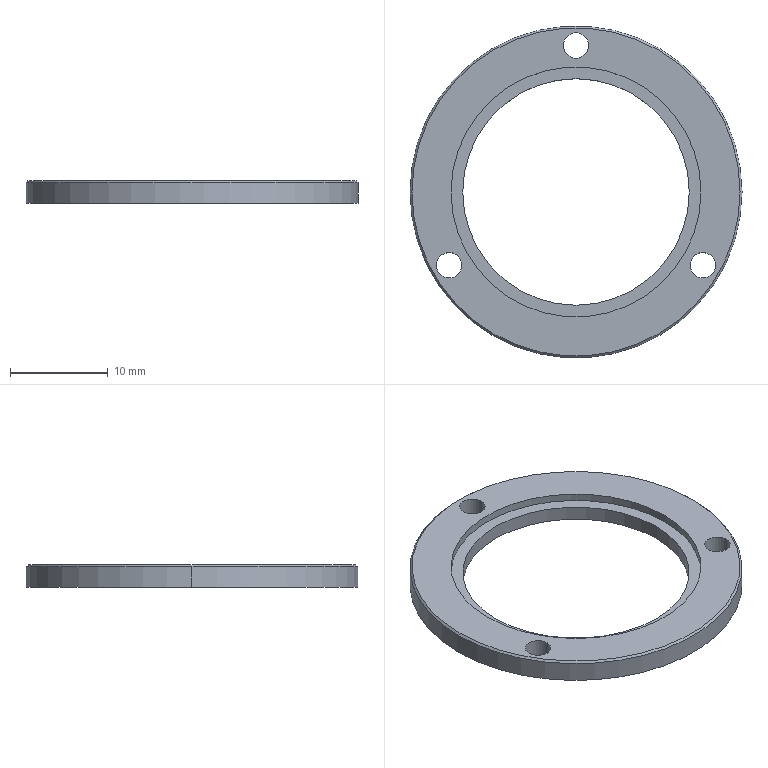Part | SolidWorks | features ICE 6, Chamfer 2, Cut 2, HoleWzd 2, MoveFace 2, Extrusion 1 | 1 solid | 17 faces | box 34 x 34 x 2.3 mm | volume 1004 mm3 | cylinder 12 | plane 3 | cone 2 | commonest cylinder face diameters 2.6 x6 23.2 x2 25.6 x2 34 x2
STEP:
#1=CARTESIAN_POINT('',(39.89,-35.7,-1.3));
#2=VERTEX_POINT('',#1);
#3=CARTESIAN_POINT('',(42.49,-35.7,-1.3));
#4=VERTEX_POINT('',#3);
#5=CARTESIAN_POINT('',(41.19,-35.7,-1.3));
#6=DIRECTION('',(0.,0.,1.));
#7=DIRECTION('',(1.,0.,0.));
#8=AXIS2_PLACEMENT_3D('',#5,#6,#7);
#9=CIRCLE('',#8,1.3);
#10=EDGE_CURVE('',#2,#4,#9,.T.);
#11=ORIENTED_EDGE('',*,*,#10,.F.);
#12=CARTESIAN_POINT('',(39.89,-35.7,1.));
#13=VERTEX_POINT('',#12);
#14=CARTESIAN_POINT('',(39.89,-35.7,-1.3));
#15=DIRECTION('',(0.,0.,1.));
#16=VECTOR('',#15,1000.);
#17=LINE('',#14,#16);
#18=EDGE_CURVE('',#2,#13,#17,.T.);
#19=ORIENTED_EDGE('',*,*,#18,.T.);
#20=CARTESIAN_POINT('',(42.49,-35.7,1.));
#21=VERTEX_POINT('',#20);
#22=CARTESIAN_POINT('',(41.19,-35.7,1.));
#23=DIRECTION('',(0.,0.,1.));
#24=DIRECTION('',(1.,0.,0.));
#25=AXIS2_PLACEMENT_3D('',#22,#23,#24);
#26=CIRCLE('',#25,1.3);
#27=EDGE_CURVE('',#13,#21,#26,.T.);
#28=ORIENTED_EDGE('',*,*,#27,.T.);
#29=CARTESIAN_POINT('',(42.49,-35.7,-1.3));
#30=DIRECTION('',(0.,0.,1.));
#31=VECTOR('',#30,1000.);
#32=LINE('',#29,#31);
#33=EDGE_CURVE('',#4,#21,#32,.T.);
#34=ORIENTED_EDGE('',*,*,#33,.F.);
#35=EDGE_LOOP('',(#11,#19,#28,#34));
#36=FACE_OUTER_BOUND('',#35,.T.);
#37=CARTESIAN_POINT('',(41.19,-35.7,-1.3));
#38=DIRECTION('',(0.,0.,1.));
#39=DIRECTION('',(1.,0.,0.));
#40=AXIS2_PLACEMENT_3D('',#37,#38,#39);
#41=CYLINDRICAL_SURFACE('',#40,1.3);
#42=ADVANCED_FACE('',(#36),#41,.F.);
#43=CARTESIAN_POINT('',(26.9,-13.2,-1.3));
#44=VERTEX_POINT('',#43);
#45=CARTESIAN_POINT('',(29.5,-13.2,-1.3));
#46=VERTEX_POINT('',#45);
#47=CARTESIAN_POINT('',(28.2,-13.2,-1.3));
#48=DIRECTION('',(0.,0.,1.));
#49=DIRECTION('',(1.,0.,0.));
#50=AXIS2_PLACEMENT_3D('',#47,#48,#49);
#51=CIRCLE('',#50,1.3);
#52=EDGE_CURVE('',#44,#46,#51,.T.);
#53=ORIENTED_EDGE('',*,*,#52,.F.);
#54=CARTESIAN_POINT('',(26.9,-13.2,1.));
#55=VERTEX_POINT('',#54);
#56=CARTESIAN_POINT('',(26.9,-13.2,-1.3));
#57=DIRECTION('',(0.,0.,1.));
#58=VECTOR('',#57,1000.);
#59=LINE('',#56,#58);
#60=EDGE_CURVE('',#44,#55,#59,.T.);
#61=ORIENTED_EDGE('',*,*,#60,.T.);
#62=CARTESIAN_POINT('',(29.5,-13.2,1.));
#63=VERTEX_POINT('',#62);
#64=CARTESIAN_POINT('',(28.2,-13.2,1.));
#65=DIRECTION('',(0.,0.,1.));
#66=DIRECTION('',(1.,0.,0.));
#67=AXIS2_PLACEMENT_3D('',#64,#65,#66);
#68=CIRCLE('',#67,1.3);
#69=EDGE_CURVE('',#55,#63,#68,.T.);
#70=ORIENTED_EDGE('',*,*,#69,.T.);
#71=CARTESIAN_POINT('',(29.5,-13.2,-1.3));
#72=DIRECTION('',(0.,0.,1.));
#73=VECTOR('',#72,1000.);
#74=LINE('',#71,#73);
#75=EDGE_CURVE('',#46,#63,#74,.T.);
#76=ORIENTED_EDGE('',*,*,#75,.F.);
#77=EDGE_LOOP('',(#53,#61,#70,#76));
#78=FACE_OUTER_BOUND('',#77,.T.);
#79=CARTESIAN_POINT('',(28.2,-13.2,-1.3));
#80=DIRECTION('',(0.,0.,1.));
#81=DIRECTION('',(1.,0.,0.));
#82=AXIS2_PLACEMENT_3D('',#79,#80,#81);
#83=CYLINDRICAL_SURFACE('',#82,1.3);
#84=ADVANCED_FACE('',(#78),#83,.F.);
#85=CARTESIAN_POINT('',(13.91,-35.7,-1.3));
#86=VERTEX_POINT('',#85);
#87=CARTESIAN_POINT('',(16.51,-35.7,-1.3));
#88=VERTEX_POINT('',#87);
#89=CARTESIAN_POINT('',(15.21,-35.7,-1.3));
#90=DIRECTION('',(0.,0.,1.));
#91=DIRECTION('',(1.,0.,0.));
#92=AXIS2_PLACEMENT_3D('',#89,#90,#91);
#93=CIRCLE('',#92,1.3);
#94=EDGE_CURVE('',#86,#88,#93,.T.);
#95=ORIENTED_EDGE('',*,*,#94,.F.);
#96=CARTESIAN_POINT('',(13.91,-35.7,1.));
#97=VERTEX_POINT('',#96);
#98=CARTESIAN_POINT('',(13.91,-35.7,-1.3));
#99=DIRECTION('',(0.,0.,1.));
#100=VECTOR('',#99,1000.);
#101=LINE('',#98,#100);
#102=EDGE_CURVE('',#86,#97,#101,.T.);
#103=ORIENTED_EDGE('',*,*,#102,.T.);
#104=CARTESIAN_POINT('',(16.51,-35.7,1.));
#105=VERTEX_POINT('',#104);
#106=CARTESIAN_POINT('',(15.21,-35.7,1.));
#107=DIRECTION('',(0.,0.,1.));
#108=DIRECTION('',(1.,0.,0.));
#109=AXIS2_PLACEMENT_3D('',#106,#107,#108);
#110=CIRCLE('',#109,1.3);
#111=EDGE_CURVE('',#97,#105,#110,.T.);
#112=ORIENTED_EDGE('',*,*,#111,.T.);
#113=CARTESIAN_POINT('',(16.51,-35.7,-1.3));
#114=DIRECTION('',(0.,0.,1.));
#115=VECTOR('',#114,1000.);
#116=LINE('',#113,#115);
#117=EDGE_CURVE('',#88,#105,#116,.T.);
#118=ORIENTED_EDGE('',*,*,#117,.F.);
#119=EDGE_LOOP('',(#95,#103,#112,#118));
#120=FACE_OUTER_BOUND('',#119,.T.);
#121=CARTESIAN_POINT('',(15.21,-35.7,-1.3));
#122=DIRECTION('',(0.,0.,1.));
#123=DIRECTION('',(1.,0.,0.));
#124=AXIS2_PLACEMENT_3D('',#121,#122,#123);
#125=CYLINDRICAL_SURFACE('',#124,1.3);
#126=ADVANCED_FACE('',(#120),#125,.F.);
#127=CARTESIAN_POINT('',(45.,-28.2,1.));
#128=VERTEX_POINT('',#127);
#129=CARTESIAN_POINT('',(11.4,-28.2,1.));
#130=VERTEX_POINT('',#129);
#131=CARTESIAN_POINT('',(28.2,-28.2,1.));
#132=DIRECTION('',(0.,0.,1.));
#133=DIRECTION('',(-1.,0.,0.));
#134=AXIS2_PLACEMENT_3D('',#131,#132,#133);
#135=CIRCLE('',#134,16.8);
#136=EDGE_CURVE('',#128,#130,#135,.T.);
#137=ORIENTED_EDGE('',*,*,#136,.F.);
#138=CARTESIAN_POINT('',(45.2,-28.2,0.8));
#139=VERTEX_POINT('',#138);
#140=CARTESIAN_POINT('',(45.2,-28.2,0.8));
#141=DIRECTION('',(0.7071,0.,-0.7071));
#142=VECTOR('',#141,1000.);
#143=LINE('',#140,#142);
#144=EDGE_CURVE('',#128,#139,#143,.T.);
#145=ORIENTED_EDGE('',*,*,#144,.T.);
#146=CARTESIAN_POINT('',(11.2,-28.2,0.8));
#147=VERTEX_POINT('',#146);
#148=CARTESIAN_POINT('',(28.2,-28.2,0.8));
#149=DIRECTION('',(0.,0.,-1.));
#150=DIRECTION('',(-1.,0.,0.));
#151=AXIS2_PLACEMENT_3D('',#148,#149,#150);
#152=CIRCLE('',#151,17.);
#153=EDGE_CURVE('',#147,#139,#152,.T.);
#154=ORIENTED_EDGE('',*,*,#153,.F.);
#155=CARTESIAN_POINT('',(11.2,-28.2,0.8));
#156=DIRECTION('',(-0.7071,0.,-0.7071));
#157=VECTOR('',#156,1000.);
#158=LINE('',#155,#157);
#159=EDGE_CURVE('',#130,#147,#158,.T.);
#160=ORIENTED_EDGE('',*,*,#159,.F.);
#161=EDGE_LOOP('',(#137,#145,#154,#160));
#162=FACE_OUTER_BOUND('',#161,.T.);
#163=CARTESIAN_POINT('',(28.2,-28.2,0.8));
#164=DIRECTION('',(0.,0.,-1.));
#165=DIRECTION('',(-1.,0.,0.));
#166=AXIS2_PLACEMENT_3D('',#163,#164,#165);
#167=CONICAL_SURFACE('',#166,17.,0.7854);
#168=ADVANCED_FACE('',(#162),#167,.T.);
#169=CARTESIAN_POINT('',(16.6,-28.2,-1.3));
#170=VERTEX_POINT('',#169);
#171=CARTESIAN_POINT('',(39.8,-28.2,-1.3));
#172=VERTEX_POINT('',#171);
#173=CARTESIAN_POINT('',(28.2,-28.2,-1.3));
#174=DIRECTION('',(0.,0.,1.));
#175=DIRECTION('',(1.,0.,0.));
#176=AXIS2_PLACEMENT_3D('',#173,#174,#175);
#177=CIRCLE('',#176,11.6);
#178=EDGE_CURVE('',#170,#172,#177,.T.);
#179=ORIENTED_EDGE('',*,*,#178,.F.);
#180=CARTESIAN_POINT('',(16.6,-28.2,0.2));
#181=VERTEX_POINT('',#180);
#182=CARTESIAN_POINT('',(16.6,-28.2,-1.3));
#183=DIRECTION('',(0.,0.,1.));
#184=VECTOR('',#183,1000.);
#185=LINE('',#182,#184);
#186=EDGE_CURVE('',#170,#181,#185,.T.);
#187=ORIENTED_EDGE('',*,*,#186,.T.);
#188=CARTESIAN_POINT('',(39.8,-28.2,0.2));
#189=VERTEX_POINT('',#188);
#190=CARTESIAN_POINT('',(28.2,-28.2,0.2));
#191=DIRECTION('',(0.,0.,1.));
#192=DIRECTION('',(1.,0.,0.));
#193=AXIS2_PLACEMENT_3D('',#190,#191,#192);
#194=CIRCLE('',#193,11.6);
#195=EDGE_CURVE('',#181,#189,#194,.T.);
#196=ORIENTED_EDGE('',*,*,#195,.T.);
#197=CARTESIAN_POINT('',(39.8,-28.2,-1.3));
#198=DIRECTION('',(0.,0.,1.));
#199=VECTOR('',#198,1000.);
#200=LINE('',#197,#199);
#201=EDGE_CURVE('',#172,#189,#200,.T.);
#202=ORIENTED_EDGE('',*,*,#201,.F.);
#203=EDGE_LOOP('',(#179,#187,#196,#202));
#204=FACE_OUTER_BOUND('',#203,.T.);
#205=CARTESIAN_POINT('',(28.2,-28.2,-1.3));
#206=DIRECTION('',(0.,0.,1.));
#207=DIRECTION('',(1.,0.,0.));
#208=AXIS2_PLACEMENT_3D('',#205,#206,#207);
#209=CYLINDRICAL_SURFACE('',#208,11.6);
#210=ADVANCED_FACE('',(#204),#209,.F.);
#211=CARTESIAN_POINT('',(15.4,-28.2,0.2));
#212=VERTEX_POINT('',#211);
#213=CARTESIAN_POINT('',(41.,-28.2,0.2));
#214=VERTEX_POINT('',#213);
#215=CARTESIAN_POINT('',(28.2,-28.2,0.2));
#216=DIRECTION('',(0.,0.,1.));
#217=DIRECTION('',(1.,0.,0.));
#218=AXIS2_PLACEMENT_3D('',#215,#216,#217);
#219=CIRCLE('',#218,12.8);
#220=EDGE_CURVE('',#212,#214,#219,.T.);
#221=ORIENTED_EDGE('',*,*,#220,.F.);
#222=CARTESIAN_POINT('',(15.4,-28.2,1.));
#223=VERTEX_POINT('',#222);
#224=CARTESIAN_POINT('',(15.4,-28.2,0.2));
#225=DIRECTION('',(0.,0.,1.));
#226=VECTOR('',#225,1000.);
#227=LINE('',#224,#226);
#228=EDGE_CURVE('',#212,#223,#227,.T.);
#229=ORIENTED_EDGE('',*,*,#228,.T.);
#230=CARTESIAN_POINT('',(41.,-28.2,1.));
#231=VERTEX_POINT('',#230);
#232=CARTESIAN_POINT('',(28.2,-28.2,1.));
#233=DIRECTION('',(0.,0.,1.));
#234=DIRECTION('',(1.,0.,0.));
#235=AXIS2_PLACEMENT_3D('',#232,#233,#234);
#236=CIRCLE('',#235,12.8);
#237=EDGE_CURVE('',#223,#231,#236,.T.);
#238=ORIENTED_EDGE('',*,*,#237,.T.);
#239=CARTESIAN_POINT('',(41.,-28.2,0.2));
#240=DIRECTION('',(0.,0.,1.));
#241=VECTOR('',#240,1000.);
#242=LINE('',#239,#241);
#243=EDGE_CURVE('',#214,#231,#242,.T.);
#244=ORIENTED_EDGE('',*,*,#243,.F.);
#245=EDGE_LOOP('',(#221,#229,#238,#244));
#246=FACE_OUTER_BOUND('',#245,.T.);
#247=CARTESIAN_POINT('',(28.2,-28.2,0.2));
#248=DIRECTION('',(0.,0.,1.));
#249=DIRECTION('',(1.,0.,0.));
#250=AXIS2_PLACEMENT_3D('',#247,#248,#249);
#251=CYLINDRICAL_SURFACE('',#250,12.8);
#252=ADVANCED_FACE('',(#246),#251,.F.);
#253=CARTESIAN_POINT('',(11.2,-28.2,-1.3));
#254=VERTEX_POINT('',#253);
#255=CARTESIAN_POINT('',(45.2,-28.2,-1.3));
#256=VERTEX_POINT('',#255);
#257=CARTESIAN_POINT('',(28.2,-28.2,-1.3));
#258=DIRECTION('',(0.,0.,-1.));
#259=DIRECTION('',(-1.,0.,0.));
#260=AXIS2_PLACEMENT_3D('',#257,#258,#259);
#261=CIRCLE('',#260,17.);
#262=EDGE_CURVE('',#254,#256,#261,.T.);
#263=ORIENTED_EDGE('',*,*,#262,.F.);
#264=CARTESIAN_POINT('',(11.2,-28.2,-5.));
#265=DIRECTION('',(0.,0.,1.));
#266=VECTOR('',#265,1000.);
#267=LINE('',#264,#266);
#268=EDGE_CURVE('',#254,#147,#267,.T.);
#269=ORIENTED_EDGE('',*,*,#268,.T.);
#270=ORIENTED_EDGE('',*,*,#153,.T.);
#271=CARTESIAN_POINT('',(45.2,-28.2,-5.));
#272=DIRECTION('',(0.,0.,1.));
#273=VECTOR('',#272,1000.);
#274=LINE('',#271,#273);
#275=EDGE_CURVE('',#256,#139,#274,.T.);
#276=ORIENTED_EDGE('',*,*,#275,.F.);
#277=EDGE_LOOP('',(#263,#269,#270,#276));
#278=FACE_OUTER_BOUND('',#277,.T.);
#279=CARTESIAN_POINT('',(28.2,-28.2,-5.));
#280=DIRECTION('',(0.,0.,1.));
#281=DIRECTION('',(1.,0.,0.));
#282=AXIS2_PLACEMENT_3D('',#279,#280,#281);
#283=CYLINDRICAL_SURFACE('',#282,17.);
#284=ADVANCED_FACE('',(#278),#283,.T.);
#285=ORIENTED_EDGE('',*,*,#268,.F.);
#286=CARTESIAN_POINT('',(28.2,-28.2,-1.3));
#287=DIRECTION('',(0.,0.,-1.));
#288=DIRECTION('',(-1.,0.,0.));
#289=AXIS2_PLACEMENT_3D('',#286,#287,#288);
#290=CIRCLE('',#289,17.);
#291=EDGE_CURVE('',#256,#254,#290,.T.);
#292=ORIENTED_EDGE('',*,*,#291,.F.);
#293=ORIENTED_EDGE('',*,*,#275,.T.);
#294=CARTESIAN_POINT('',(28.2,-28.2,0.8));
#295=DIRECTION('',(0.,0.,-1.));
#296=DIRECTION('',(-1.,0.,0.));
#297=AXIS2_PLACEMENT_3D('',#294,#295,#296);
#298=CIRCLE('',#297,17.);
#299=EDGE_CURVE('',#139,#147,#298,.T.);
#300=ORIENTED_EDGE('',*,*,#299,.T.);
#301=EDGE_LOOP('',(#285,#292,#293,#300));
#302=FACE_OUTER_BOUND('',#301,.T.);
#303=CARTESIAN_POINT('',(28.2,-28.2,-5.));
#304=DIRECTION('',(0.,0.,1.));
#305=DIRECTION('',(1.,0.,0.));
#306=AXIS2_PLACEMENT_3D('',#303,#304,#305);
#307=CYLINDRICAL_SURFACE('',#306,17.);
#308=ADVANCED_FACE('',(#302),#307,.T.);
#309=CARTESIAN_POINT('',(41.19,-35.7,1.));
#310=DIRECTION('',(0.,0.,1.));
#311=DIRECTION('',(1.,0.,0.));
#312=AXIS2_PLACEMENT_3D('',#309,#310,#311);
#313=CIRCLE('',#312,1.3);
#314=EDGE_CURVE('',#21,#13,#313,.T.);
#315=ORIENTED_EDGE('',*,*,#314,.F.);
#316=ORIENTED_EDGE('',*,*,#27,.F.);
#317=EDGE_LOOP('',(#315,#316));
#318=FACE_BOUND('',#317,.T.);
#319=CARTESIAN_POINT('',(28.2,-13.2,1.));
#320=DIRECTION('',(0.,0.,1.));
#321=DIRECTION('',(1.,0.,0.));
#322=AXIS2_PLACEMENT_3D('',#319,#320,#321);
#323=CIRCLE('',#322,1.3);
#324=EDGE_CURVE('',#63,#55,#323,.T.);
#325=ORIENTED_EDGE('',*,*,#324,.F.);
#326=ORIENTED_EDGE('',*,*,#69,.F.);
#327=EDGE_LOOP('',(#325,#326));
#328=FACE_BOUND('',#327,.T.);
#329=CARTESIAN_POINT('',(15.21,-35.7,1.));
#330=DIRECTION('',(0.,0.,1.));
#331=DIRECTION('',(1.,0.,0.));
#332=AXIS2_PLACEMENT_3D('',#329,#330,#331);
#333=CIRCLE('',#332,1.3);
#334=EDGE_CURVE('',#105,#97,#333,.T.);
#335=ORIENTED_EDGE('',*,*,#334,.F.);
#336=ORIENTED_EDGE('',*,*,#111,.F.);
#337=EDGE_LOOP('',(#335,#336));
#338=FACE_BOUND('',#337,.T.);
#339=CARTESIAN_POINT('',(28.2,-28.2,1.));
#340=DIRECTION('',(0.,0.,1.));
#341=DIRECTION('',(-1.,0.,0.));
#342=AXIS2_PLACEMENT_3D('',#339,#340,#341);
#343=CIRCLE('',#342,16.8);
#344=EDGE_CURVE('',#130,#128,#343,.T.);
#345=ORIENTED_EDGE('',*,*,#344,.T.);
#346=ORIENTED_EDGE('',*,*,#136,.T.);
#347=EDGE_LOOP('',(#345,#346));
#348=FACE_OUTER_BOUND('',#347,.T.);
#349=CARTESIAN_POINT('',(28.2,-28.2,1.));
#350=DIRECTION('',(0.,0.,1.));
#351=DIRECTION('',(1.,0.,0.));
#352=AXIS2_PLACEMENT_3D('',#349,#350,#351);
#353=CIRCLE('',#352,12.8);
#354=EDGE_CURVE('',#231,#223,#353,.T.);
#355=ORIENTED_EDGE('',*,*,#354,.F.);
#356=ORIENTED_EDGE('',*,*,#237,.F.);
#357=EDGE_LOOP('',(#355,#356));
#358=FACE_BOUND('',#357,.T.);
#359=CARTESIAN_POINT('',(28.2,-28.2,1.));
#360=DIRECTION('',(0.,0.,-1.));
#361=DIRECTION('',(-1.,0.,0.));
#362=AXIS2_PLACEMENT_3D('',#359,#360,#361);
#363=PLANE('',#362);
#364=ADVANCED_FACE('',(#318,#328,#338,#348,#358),#363,.F.);
#365=CARTESIAN_POINT('',(28.2,-28.2,0.2));
#366=DIRECTION('',(0.,0.,1.));
#367=DIRECTION('',(1.,0.,0.));
#368=AXIS2_PLACEMENT_3D('',#365,#366,#367);
#369=CIRCLE('',#368,12.8);
#370=EDGE_CURVE('',#214,#212,#369,.T.);
#371=ORIENTED_EDGE('',*,*,#370,.T.);
#372=ORIENTED_EDGE('',*,*,#220,.T.);
#373=EDGE_LOOP('',(#371,#372));
#374=FACE_OUTER_BOUND('',#373,.T.);
#375=CARTESIAN_POINT('',(28.2,-28.2,0.2));
#376=DIRECTION('',(0.,0.,1.));
#377=DIRECTION('',(1.,0.,0.));
#378=AXIS2_PLACEMENT_3D('',#375,#376,#377);
#379=CIRCLE('',#378,11.6);
#380=EDGE_CURVE('',#189,#181,#379,.T.);
#381=ORIENTED_EDGE('',*,*,#380,.F.);
#382=ORIENTED_EDGE('',*,*,#195,.F.);
#383=EDGE_LOOP('',(#381,#382));
#384=FACE_BOUND('',#383,.T.);
#385=CARTESIAN_POINT('',(28.2,-28.2,0.2));
#386=DIRECTION('',(0.,0.,1.));
#387=DIRECTION('',(1.,0.,0.));
#388=AXIS2_PLACEMENT_3D('',#385,#386,#387);
#389=PLANE('',#388);
#390=ADVANCED_FACE('',(#374,#384),#389,.T.);
#391=ORIENTED_EDGE('',*,*,#228,.F.);
#392=ORIENTED_EDGE('',*,*,#370,.F.);
#393=ORIENTED_EDGE('',*,*,#243,.T.);
#394=ORIENTED_EDGE('',*,*,#354,.T.);
#395=EDGE_LOOP('',(#391,#392,#393,#394));
#396=FACE_OUTER_BOUND('',#395,.T.);
#397=CARTESIAN_POINT('',(28.2,-28.2,0.2));
#398=DIRECTION('',(0.,0.,1.));
#399=DIRECTION('',(1.,0.,0.));
#400=AXIS2_PLACEMENT_3D('',#397,#398,#399);
#401=CYLINDRICAL_SURFACE('',#400,12.8);
#402=ADVANCED_FACE('',(#396),#401,.F.);
#403=CARTESIAN_POINT('',(41.19,-35.7,-1.3));
#404=DIRECTION('',(0.,0.,1.));
#405=DIRECTION('',(1.,0.,0.));
#406=AXIS2_PLACEMENT_3D('',#403,#404,#405);
#407=CIRCLE('',#406,1.3);
#408=EDGE_CURVE('',#4,#2,#407,.T.);
#409=ORIENTED_EDGE('',*,*,#408,.T.);
#410=ORIENTED_EDGE('',*,*,#10,.T.);
#411=EDGE_LOOP('',(#409,#410));
#412=FACE_BOUND('',#411,.T.);
#413=CARTESIAN_POINT('',(28.2,-13.2,-1.3));
#414=DIRECTION('',(0.,0.,1.));
#415=DIRECTION('',(1.,0.,0.));
#416=AXIS2_PLACEMENT_3D('',#413,#414,#415);
#417=CIRCLE('',#416,1.3);
#418=EDGE_CURVE('',#46,#44,#417,.T.);
#419=ORIENTED_EDGE('',*,*,#418,.T.);
#420=ORIENTED_EDGE('',*,*,#52,.T.);
#421=EDGE_LOOP('',(#419,#420));
#422=FACE_BOUND('',#421,.T.);
#423=CARTESIAN_POINT('',(15.21,-35.7,-1.3));
#424=DIRECTION('',(0.,0.,1.));
#425=DIRECTION('',(1.,0.,0.));
#426=AXIS2_PLACEMENT_3D('',#423,#424,#425);
#427=CIRCLE('',#426,1.3);
#428=EDGE_CURVE('',#88,#86,#427,.T.);
#429=ORIENTED_EDGE('',*,*,#428,.T.);
#430=ORIENTED_EDGE('',*,*,#94,.T.);
#431=EDGE_LOOP('',(#429,#430));
#432=FACE_BOUND('',#431,.T.);
#433=CARTESIAN_POINT('',(28.2,-28.2,-1.3));
#434=DIRECTION('',(0.,0.,1.));
#435=DIRECTION('',(1.,0.,0.));
#436=AXIS2_PLACEMENT_3D('',#433,#434,#435);
#437=CIRCLE('',#436,11.6);
#438=EDGE_CURVE('',#172,#170,#437,.T.);
#439=ORIENTED_EDGE('',*,*,#438,.T.);
#440=ORIENTED_EDGE('',*,*,#178,.T.);
#441=EDGE_LOOP('',(#439,#440));
#442=FACE_BOUND('',#441,.T.);
#443=ORIENTED_EDGE('',*,*,#291,.T.);
#444=ORIENTED_EDGE('',*,*,#262,.T.);
#445=EDGE_LOOP('',(#443,#444));
#446=FACE_OUTER_BOUND('',#445,.T.);
#447=CARTESIAN_POINT('',(28.2,-28.2,-1.3));
#448=DIRECTION('',(0.,0.,1.));
#449=DIRECTION('',(1.,0.,0.));
#450=AXIS2_PLACEMENT_3D('',#447,#448,#449);
#451=PLANE('',#450);
#452=ADVANCED_FACE('',(#412,#422,#432,#442,#446),#451,.F.);
#453=ORIENTED_EDGE('',*,*,#186,.F.);
#454=ORIENTED_EDGE('',*,*,#438,.F.);
#455=ORIENTED_EDGE('',*,*,#201,.T.);
#456=ORIENTED_EDGE('',*,*,#380,.T.);
#457=EDGE_LOOP('',(#453,#454,#455,#456));
#458=FACE_OUTER_BOUND('',#457,.T.);
#459=CARTESIAN_POINT('',(28.2,-28.2,-1.3));
#460=DIRECTION('',(0.,0.,1.));
#461=DIRECTION('',(1.,0.,0.));
#462=AXIS2_PLACEMENT_3D('',#459,#460,#461);
#463=CYLINDRICAL_SURFACE('',#462,11.6);
#464=ADVANCED_FACE('',(#458),#463,.F.);
#465=ORIENTED_EDGE('',*,*,#144,.F.);
#466=ORIENTED_EDGE('',*,*,#344,.F.);
#467=ORIENTED_EDGE('',*,*,#159,.T.);
#468=ORIENTED_EDGE('',*,*,#299,.F.);
#469=EDGE_LOOP('',(#465,#466,#467,#468));
#470=FACE_OUTER_BOUND('',#469,.T.);
#471=CARTESIAN_POINT('',(28.2,-28.2,0.8));
#472=DIRECTION('',(0.,0.,-1.));
#473=DIRECTION('',(-1.,0.,0.));
#474=AXIS2_PLACEMENT_3D('',#471,#472,#473);
#475=CONICAL_SURFACE('',#474,17.,0.7854);
#476=ADVANCED_FACE('',(#470),#475,.T.);
#477=ORIENTED_EDGE('',*,*,#102,.F.);
#478=ORIENTED_EDGE('',*,*,#428,.F.);
#479=ORIENTED_EDGE('',*,*,#117,.T.);
#480=ORIENTED_EDGE('',*,*,#334,.T.);
#481=EDGE_LOOP('',(#477,#478,#479,#480));
#482=FACE_OUTER_BOUND('',#481,.T.);
#483=CARTESIAN_POINT('',(15.21,-35.7,-1.3));
#484=DIRECTION('',(0.,0.,1.));
#485=DIRECTION('',(1.,0.,0.));
#486=AXIS2_PLACEMENT_3D('',#483,#484,#485);
#487=CYLINDRICAL_SURFACE('',#486,1.3);
#488=ADVANCED_FACE('',(#482),#487,.F.);
#489=ORIENTED_EDGE('',*,*,#60,.F.);
#490=ORIENTED_EDGE('',*,*,#418,.F.);
#491=ORIENTED_EDGE('',*,*,#75,.T.);
#492=ORIENTED_EDGE('',*,*,#324,.T.);
#493=EDGE_LOOP('',(#489,#490,#491,#492));
#494=FACE_OUTER_BOUND('',#493,.T.);
#495=CARTESIAN_POINT('',(28.2,-13.2,-1.3));
#496=DIRECTION('',(0.,0.,1.));
#497=DIRECTION('',(1.,0.,0.));
#498=AXIS2_PLACEMENT_3D('',#495,#496,#497);
#499=CYLINDRICAL_SURFACE('',#498,1.3);
#500=ADVANCED_FACE('',(#494),#499,.F.);
#501=ORIENTED_EDGE('',*,*,#18,.F.);
#502=ORIENTED_EDGE('',*,*,#408,.F.);
#503=ORIENTED_EDGE('',*,*,#33,.T.);
#504=ORIENTED_EDGE('',*,*,#314,.T.);
#505=EDGE_LOOP('',(#501,#502,#503,#504));
#506=FACE_OUTER_BOUND('',#505,.T.);
#507=CARTESIAN_POINT('',(41.19,-35.7,-1.3));
#508=DIRECTION('',(0.,0.,1.));
#509=DIRECTION('',(1.,0.,0.));
#510=AXIS2_PLACEMENT_3D('',#507,#508,#509);
#511=CYLINDRICAL_SURFACE('',#510,1.3);
#512=ADVANCED_FACE('',(#506),#511,.F.);
#513=CLOSED_SHELL('',(#42,#84,#126,#168,#210,#252,#284,#308,#364,#390,#402,#452,#464,#476,#488,#500,#512));
#514=MANIFOLD_SOLID_BREP('',#513);
#515=CARTESIAN_POINT('',(0.,0.,0.));
#516=DIRECTION('',(0.,0.,1.));
#517=DIRECTION('',(1.,0.,0.));
#518=AXIS2_PLACEMENT_3D('',#515,#516,#517);
#519=(LENGTH_UNIT()NAMED_UNIT(*)SI_UNIT(.MILLI.,.METRE.));
#520=UNCERTAINTY_MEASURE_WITH_UNIT(LENGTH_MEASURE(0.00001),#519,'','');
#521=(NAMED_UNIT(*)PLANE_ANGLE_UNIT()SI_UNIT($,.RADIAN.));
#522=(NAMED_UNIT(*)SI_UNIT($,.STERADIAN.)SOLID_ANGLE_UNIT());
#523=(GEOMETRIC_REPRESENTATION_CONTEXT(3)GLOBAL_UNCERTAINTY_ASSIGNED_CONTEXT((#520))GLOBAL_UNIT_ASSIGNED_CONTEXT((#519,#521,#522))REPRESENTATION_CONTEXT('',''));
#524=ADVANCED_BREP_SHAPE_REPRESENTATION('',(#514,#518),#523);